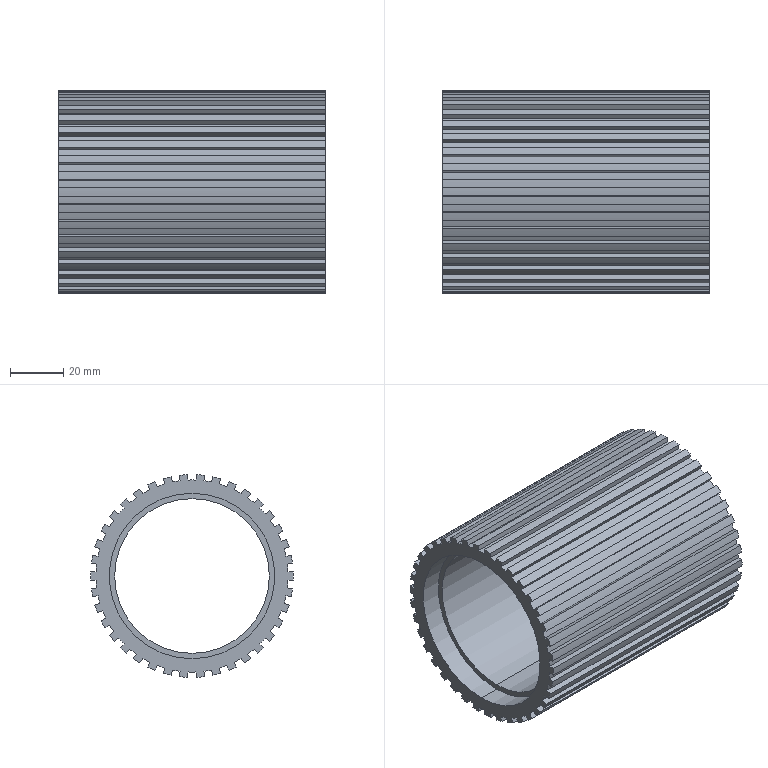Part | SolidWorks | features BaseBody 1 | 1 solid | 163 faces | box 100 x 76 x 75.929 mm | volume 159717 mm3 | cylinder 83 | plane 80 | commonest cylinder face diameters 72 x39 76 x38 62 x4 58 x2